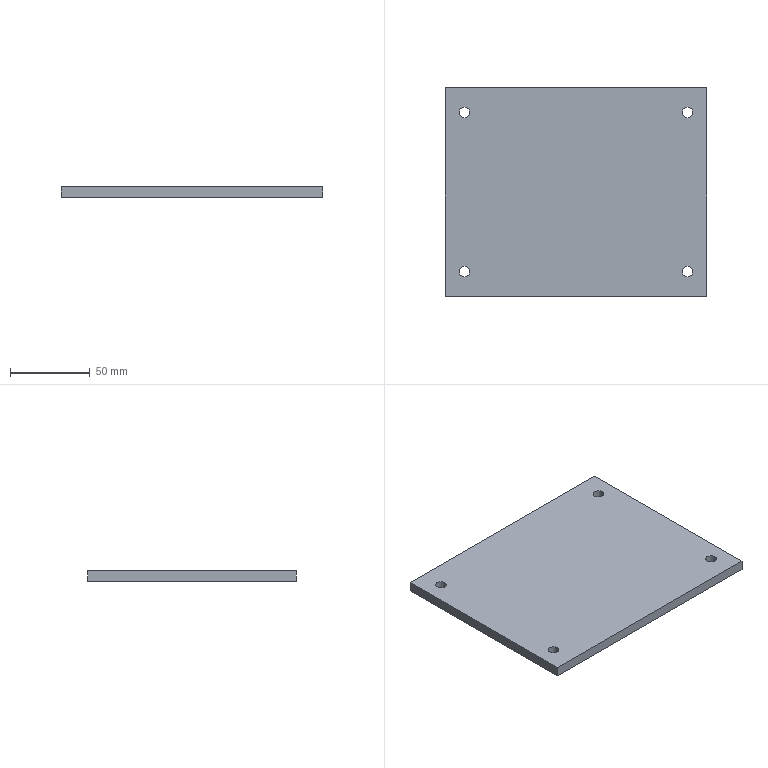Part | SolidWorks | features BaseBody 1 | 1 solid | 14 faces | box 164 x 131 x 6.4 mm | volume 136609 mm3 | cylinder 8 | plane 6 | commonest cylinder face diameters 6.647 x8
STEP:
#1=CARTESIAN_POINT('',(3.323,99.5,0.));
#2=VERTEX_POINT('',#1);
#3=CARTESIAN_POINT('',(-3.324,99.5,0.));
#4=VERTEX_POINT('',#3);
#5=CARTESIAN_POINT('',(0.,99.5,0.));
#6=DIRECTION('',(0.,0.,-1.));
#7=DIRECTION('',(1.,0.,0.));
#8=AXIS2_PLACEMENT_3D('',#5,#6,#7);
#9=CIRCLE('',#8,3.324);
#10=EDGE_CURVE('',#2,#4,#9,.T.);
#11=ORIENTED_EDGE('',*,*,#10,.T.);
#12=CARTESIAN_POINT('',(-3.324,99.5,6.4));
#13=VERTEX_POINT('',#12);
#14=CARTESIAN_POINT('',(-3.324,99.5,-203.595));
#15=DIRECTION('',(0.,0.,1.));
#16=VECTOR('',#15,1000.);
#17=LINE('',#14,#16);
#18=EDGE_CURVE('',#4,#13,#17,.T.);
#19=ORIENTED_EDGE('',*,*,#18,.T.);
#20=CARTESIAN_POINT('',(3.323,99.5,6.4));
#21=VERTEX_POINT('',#20);
#22=CARTESIAN_POINT('',(0.,99.5,6.4));
#23=DIRECTION('',(0.,0.,-1.));
#24=DIRECTION('',(1.,0.,0.));
#25=AXIS2_PLACEMENT_3D('',#22,#23,#24);
#26=CIRCLE('',#25,3.324);
#27=EDGE_CURVE('',#21,#13,#26,.T.);
#28=ORIENTED_EDGE('',*,*,#27,.F.);
#29=CARTESIAN_POINT('',(3.323,99.5,-203.595));
#30=DIRECTION('',(0.,0.,1.));
#31=VECTOR('',#30,1000.);
#32=LINE('',#29,#31);
#33=EDGE_CURVE('',#2,#21,#32,.T.);
#34=ORIENTED_EDGE('',*,*,#33,.F.);
#35=EDGE_LOOP('',(#11,#19,#28,#34));
#36=FACE_OUTER_BOUND('',#35,.T.);
#37=CARTESIAN_POINT('',(0.,99.5,-203.595));
#38=DIRECTION('',(0.,0.,1.));
#39=DIRECTION('',(1.,0.,0.));
#40=AXIS2_PLACEMENT_3D('',#37,#38,#39);
#41=CYLINDRICAL_SURFACE('',#40,3.324);
#42=ADVANCED_FACE('',(#36),#41,.F.);
#43=CARTESIAN_POINT('',(3.323,-0.5,0.));
#44=VERTEX_POINT('',#43);
#45=CARTESIAN_POINT('',(-3.324,-0.5,0.));
#46=VERTEX_POINT('',#45);
#47=CARTESIAN_POINT('',(0.,-0.5,0.));
#48=DIRECTION('',(0.,0.,-1.));
#49=DIRECTION('',(1.,0.,0.));
#50=AXIS2_PLACEMENT_3D('',#47,#48,#49);
#51=CIRCLE('',#50,3.324);
#52=EDGE_CURVE('',#44,#46,#51,.T.);
#53=ORIENTED_EDGE('',*,*,#52,.T.);
#54=CARTESIAN_POINT('',(-3.324,-0.5,6.4));
#55=VERTEX_POINT('',#54);
#56=CARTESIAN_POINT('',(-3.324,-0.5,-203.595));
#57=DIRECTION('',(0.,0.,1.));
#58=VECTOR('',#57,1000.);
#59=LINE('',#56,#58);
#60=EDGE_CURVE('',#46,#55,#59,.T.);
#61=ORIENTED_EDGE('',*,*,#60,.T.);
#62=CARTESIAN_POINT('',(3.323,-0.5,6.4));
#63=VERTEX_POINT('',#62);
#64=CARTESIAN_POINT('',(0.,-0.5,6.4));
#65=DIRECTION('',(0.,0.,-1.));
#66=DIRECTION('',(1.,0.,0.));
#67=AXIS2_PLACEMENT_3D('',#64,#65,#66);
#68=CIRCLE('',#67,3.324);
#69=EDGE_CURVE('',#63,#55,#68,.T.);
#70=ORIENTED_EDGE('',*,*,#69,.F.);
#71=CARTESIAN_POINT('',(3.323,-0.5,-203.595));
#72=DIRECTION('',(0.,0.,1.));
#73=VECTOR('',#72,1000.);
#74=LINE('',#71,#73);
#75=EDGE_CURVE('',#44,#63,#74,.T.);
#76=ORIENTED_EDGE('',*,*,#75,.F.);
#77=EDGE_LOOP('',(#53,#61,#70,#76));
#78=FACE_OUTER_BOUND('',#77,.T.);
#79=CARTESIAN_POINT('',(0.,-0.5,-203.595));
#80=DIRECTION('',(0.,0.,1.));
#81=DIRECTION('',(1.,0.,0.));
#82=AXIS2_PLACEMENT_3D('',#79,#80,#81);
#83=CYLINDRICAL_SURFACE('',#82,3.324);
#84=ADVANCED_FACE('',(#78),#83,.F.);
#85=CARTESIAN_POINT('',(143.324,-0.5,0.));
#86=VERTEX_POINT('',#85);
#87=CARTESIAN_POINT('',(136.677,-0.5,0.));
#88=VERTEX_POINT('',#87);
#89=CARTESIAN_POINT('',(140.,-0.5,0.));
#90=DIRECTION('',(0.,0.,-1.));
#91=DIRECTION('',(1.,0.,0.));
#92=AXIS2_PLACEMENT_3D('',#89,#90,#91);
#93=CIRCLE('',#92,3.324);
#94=EDGE_CURVE('',#86,#88,#93,.T.);
#95=ORIENTED_EDGE('',*,*,#94,.T.);
#96=CARTESIAN_POINT('',(136.677,-0.5,6.4));
#97=VERTEX_POINT('',#96);
#98=CARTESIAN_POINT('',(136.677,-0.5,-203.595));
#99=DIRECTION('',(0.,0.,1.));
#100=VECTOR('',#99,1000.);
#101=LINE('',#98,#100);
#102=EDGE_CURVE('',#88,#97,#101,.T.);
#103=ORIENTED_EDGE('',*,*,#102,.T.);
#104=CARTESIAN_POINT('',(143.324,-0.5,6.4));
#105=VERTEX_POINT('',#104);
#106=CARTESIAN_POINT('',(140.,-0.5,6.4));
#107=DIRECTION('',(0.,0.,-1.));
#108=DIRECTION('',(1.,0.,0.));
#109=AXIS2_PLACEMENT_3D('',#106,#107,#108);
#110=CIRCLE('',#109,3.324);
#111=EDGE_CURVE('',#105,#97,#110,.T.);
#112=ORIENTED_EDGE('',*,*,#111,.F.);
#113=CARTESIAN_POINT('',(143.324,-0.5,-203.595));
#114=DIRECTION('',(0.,0.,1.));
#115=VECTOR('',#114,1000.);
#116=LINE('',#113,#115);
#117=EDGE_CURVE('',#86,#105,#116,.T.);
#118=ORIENTED_EDGE('',*,*,#117,.F.);
#119=EDGE_LOOP('',(#95,#103,#112,#118));
#120=FACE_OUTER_BOUND('',#119,.T.);
#121=CARTESIAN_POINT('',(140.,-0.5,-203.595));
#122=DIRECTION('',(0.,0.,1.));
#123=DIRECTION('',(1.,0.,0.));
#124=AXIS2_PLACEMENT_3D('',#121,#122,#123);
#125=CYLINDRICAL_SURFACE('',#124,3.324);
#126=ADVANCED_FACE('',(#120),#125,.F.);
#127=CARTESIAN_POINT('',(143.324,99.5,0.));
#128=VERTEX_POINT('',#127);
#129=CARTESIAN_POINT('',(136.677,99.5,0.));
#130=VERTEX_POINT('',#129);
#131=CARTESIAN_POINT('',(140.,99.5,0.));
#132=DIRECTION('',(0.,0.,-1.));
#133=DIRECTION('',(1.,0.,0.));
#134=AXIS2_PLACEMENT_3D('',#131,#132,#133);
#135=CIRCLE('',#134,3.324);
#136=EDGE_CURVE('',#128,#130,#135,.T.);
#137=ORIENTED_EDGE('',*,*,#136,.T.);
#138=CARTESIAN_POINT('',(136.677,99.5,6.4));
#139=VERTEX_POINT('',#138);
#140=CARTESIAN_POINT('',(136.677,99.5,-203.595));
#141=DIRECTION('',(0.,0.,1.));
#142=VECTOR('',#141,1000.);
#143=LINE('',#140,#142);
#144=EDGE_CURVE('',#130,#139,#143,.T.);
#145=ORIENTED_EDGE('',*,*,#144,.T.);
#146=CARTESIAN_POINT('',(143.324,99.5,6.4));
#147=VERTEX_POINT('',#146);
#148=CARTESIAN_POINT('',(140.,99.5,6.4));
#149=DIRECTION('',(0.,0.,-1.));
#150=DIRECTION('',(1.,0.,0.));
#151=AXIS2_PLACEMENT_3D('',#148,#149,#150);
#152=CIRCLE('',#151,3.324);
#153=EDGE_CURVE('',#147,#139,#152,.T.);
#154=ORIENTED_EDGE('',*,*,#153,.F.);
#155=CARTESIAN_POINT('',(143.324,99.5,-203.595));
#156=DIRECTION('',(0.,0.,1.));
#157=VECTOR('',#156,1000.);
#158=LINE('',#155,#157);
#159=EDGE_CURVE('',#128,#147,#158,.T.);
#160=ORIENTED_EDGE('',*,*,#159,.F.);
#161=EDGE_LOOP('',(#137,#145,#154,#160));
#162=FACE_OUTER_BOUND('',#161,.T.);
#163=CARTESIAN_POINT('',(140.,99.5,-203.595));
#164=DIRECTION('',(0.,0.,1.));
#165=DIRECTION('',(1.,0.,0.));
#166=AXIS2_PLACEMENT_3D('',#163,#164,#165);
#167=CYLINDRICAL_SURFACE('',#166,3.324);
#168=ADVANCED_FACE('',(#162),#167,.F.);
#169=ORIENTED_EDGE('',*,*,#10,.F.);
#170=CARTESIAN_POINT('',(0.,99.5,0.));
#171=DIRECTION('',(0.,0.,-1.));
#172=DIRECTION('',(1.,0.,0.));
#173=AXIS2_PLACEMENT_3D('',#170,#171,#172);
#174=CIRCLE('',#173,3.324);
#175=EDGE_CURVE('',#4,#2,#174,.T.);
#176=ORIENTED_EDGE('',*,*,#175,.F.);
#177=EDGE_LOOP('',(#169,#176));
#178=FACE_BOUND('',#177,.T.);
#179=ORIENTED_EDGE('',*,*,#52,.F.);
#180=CARTESIAN_POINT('',(0.,-0.5,0.));
#181=DIRECTION('',(0.,0.,-1.));
#182=DIRECTION('',(1.,0.,0.));
#183=AXIS2_PLACEMENT_3D('',#180,#181,#182);
#184=CIRCLE('',#183,3.324);
#185=EDGE_CURVE('',#46,#44,#184,.T.);
#186=ORIENTED_EDGE('',*,*,#185,.F.);
#187=EDGE_LOOP('',(#179,#186));
#188=FACE_BOUND('',#187,.T.);
#189=ORIENTED_EDGE('',*,*,#94,.F.);
#190=CARTESIAN_POINT('',(140.,-0.5,0.));
#191=DIRECTION('',(0.,0.,-1.));
#192=DIRECTION('',(1.,0.,0.));
#193=AXIS2_PLACEMENT_3D('',#190,#191,#192);
#194=CIRCLE('',#193,3.324);
#195=EDGE_CURVE('',#88,#86,#194,.T.);
#196=ORIENTED_EDGE('',*,*,#195,.F.);
#197=EDGE_LOOP('',(#189,#196));
#198=FACE_BOUND('',#197,.T.);
#199=ORIENTED_EDGE('',*,*,#136,.F.);
#200=CARTESIAN_POINT('',(140.,99.5,0.));
#201=DIRECTION('',(0.,0.,-1.));
#202=DIRECTION('',(1.,0.,0.));
#203=AXIS2_PLACEMENT_3D('',#200,#201,#202);
#204=CIRCLE('',#203,3.324);
#205=EDGE_CURVE('',#130,#128,#204,.T.);
#206=ORIENTED_EDGE('',*,*,#205,.F.);
#207=EDGE_LOOP('',(#199,#206));
#208=FACE_BOUND('',#207,.T.);
#209=CARTESIAN_POINT('',(152.,-16.,0.));
#210=VERTEX_POINT('',#209);
#211=CARTESIAN_POINT('',(152.,115.,0.));
#212=VERTEX_POINT('',#211);
#213=CARTESIAN_POINT('',(152.,49.5,0.));
#214=DIRECTION('',(0.,1.,0.));
#215=VECTOR('',#214,1000.);
#216=LINE('',#213,#215);
#217=EDGE_CURVE('',#210,#212,#216,.T.);
#218=ORIENTED_EDGE('',*,*,#217,.F.);
#219=CARTESIAN_POINT('',(-12.,-16.,0.));
#220=VERTEX_POINT('',#219);
#221=CARTESIAN_POINT('',(70.,-16.,0.));
#222=DIRECTION('',(1.,0.,0.));
#223=VECTOR('',#222,1000.);
#224=LINE('',#221,#223);
#225=EDGE_CURVE('',#220,#210,#224,.T.);
#226=ORIENTED_EDGE('',*,*,#225,.F.);
#227=CARTESIAN_POINT('',(-12.,115.,0.));
#228=VERTEX_POINT('',#227);
#229=CARTESIAN_POINT('',(-12.,49.5,0.));
#230=DIRECTION('',(0.,-1.,0.));
#231=VECTOR('',#230,1000.);
#232=LINE('',#229,#231);
#233=EDGE_CURVE('',#228,#220,#232,.T.);
#234=ORIENTED_EDGE('',*,*,#233,.F.);
#235=CARTESIAN_POINT('',(70.,115.,0.));
#236=DIRECTION('',(-1.,0.,0.));
#237=VECTOR('',#236,1000.);
#238=LINE('',#235,#237);
#239=EDGE_CURVE('',#212,#228,#238,.T.);
#240=ORIENTED_EDGE('',*,*,#239,.F.);
#241=EDGE_LOOP('',(#218,#226,#234,#240));
#242=FACE_OUTER_BOUND('',#241,.T.);
#243=CARTESIAN_POINT('',(70.,49.5,0.));
#244=DIRECTION('',(0.,0.,1.));
#245=DIRECTION('',(1.,0.,0.));
#246=AXIS2_PLACEMENT_3D('',#243,#244,#245);
#247=PLANE('',#246);
#248=ADVANCED_FACE('',(#178,#188,#198,#208,#242),#247,.F.);
#249=ORIENTED_EDGE('',*,*,#18,.F.);
#250=ORIENTED_EDGE('',*,*,#175,.T.);
#251=ORIENTED_EDGE('',*,*,#33,.T.);
#252=CARTESIAN_POINT('',(0.,99.5,6.4));
#253=DIRECTION('',(0.,0.,-1.));
#254=DIRECTION('',(1.,0.,0.));
#255=AXIS2_PLACEMENT_3D('',#252,#253,#254);
#256=CIRCLE('',#255,3.324);
#257=EDGE_CURVE('',#13,#21,#256,.T.);
#258=ORIENTED_EDGE('',*,*,#257,.F.);
#259=EDGE_LOOP('',(#249,#250,#251,#258));
#260=FACE_OUTER_BOUND('',#259,.T.);
#261=CARTESIAN_POINT('',(0.,99.5,-203.595));
#262=DIRECTION('',(0.,0.,1.));
#263=DIRECTION('',(1.,0.,0.));
#264=AXIS2_PLACEMENT_3D('',#261,#262,#263);
#265=CYLINDRICAL_SURFACE('',#264,3.324);
#266=ADVANCED_FACE('',(#260),#265,.F.);
#267=ORIENTED_EDGE('',*,*,#60,.F.);
#268=ORIENTED_EDGE('',*,*,#185,.T.);
#269=ORIENTED_EDGE('',*,*,#75,.T.);
#270=CARTESIAN_POINT('',(0.,-0.5,6.4));
#271=DIRECTION('',(0.,0.,-1.));
#272=DIRECTION('',(1.,0.,0.));
#273=AXIS2_PLACEMENT_3D('',#270,#271,#272);
#274=CIRCLE('',#273,3.324);
#275=EDGE_CURVE('',#55,#63,#274,.T.);
#276=ORIENTED_EDGE('',*,*,#275,.F.);
#277=EDGE_LOOP('',(#267,#268,#269,#276));
#278=FACE_OUTER_BOUND('',#277,.T.);
#279=CARTESIAN_POINT('',(0.,-0.5,-203.595));
#280=DIRECTION('',(0.,0.,1.));
#281=DIRECTION('',(1.,0.,0.));
#282=AXIS2_PLACEMENT_3D('',#279,#280,#281);
#283=CYLINDRICAL_SURFACE('',#282,3.324);
#284=ADVANCED_FACE('',(#278),#283,.F.);
#285=ORIENTED_EDGE('',*,*,#102,.F.);
#286=ORIENTED_EDGE('',*,*,#195,.T.);
#287=ORIENTED_EDGE('',*,*,#117,.T.);
#288=CARTESIAN_POINT('',(140.,-0.5,6.4));
#289=DIRECTION('',(0.,0.,-1.));
#290=DIRECTION('',(1.,0.,0.));
#291=AXIS2_PLACEMENT_3D('',#288,#289,#290);
#292=CIRCLE('',#291,3.324);
#293=EDGE_CURVE('',#97,#105,#292,.T.);
#294=ORIENTED_EDGE('',*,*,#293,.F.);
#295=EDGE_LOOP('',(#285,#286,#287,#294));
#296=FACE_OUTER_BOUND('',#295,.T.);
#297=CARTESIAN_POINT('',(140.,-0.5,-203.595));
#298=DIRECTION('',(0.,0.,1.));
#299=DIRECTION('',(1.,0.,0.));
#300=AXIS2_PLACEMENT_3D('',#297,#298,#299);
#301=CYLINDRICAL_SURFACE('',#300,3.324);
#302=ADVANCED_FACE('',(#296),#301,.F.);
#303=ORIENTED_EDGE('',*,*,#144,.F.);
#304=ORIENTED_EDGE('',*,*,#205,.T.);
#305=ORIENTED_EDGE('',*,*,#159,.T.);
#306=CARTESIAN_POINT('',(140.,99.5,6.4));
#307=DIRECTION('',(0.,0.,-1.));
#308=DIRECTION('',(1.,0.,0.));
#309=AXIS2_PLACEMENT_3D('',#306,#307,#308);
#310=CIRCLE('',#309,3.324);
#311=EDGE_CURVE('',#139,#147,#310,.T.);
#312=ORIENTED_EDGE('',*,*,#311,.F.);
#313=EDGE_LOOP('',(#303,#304,#305,#312));
#314=FACE_OUTER_BOUND('',#313,.T.);
#315=CARTESIAN_POINT('',(140.,99.5,-203.595));
#316=DIRECTION('',(0.,0.,1.));
#317=DIRECTION('',(1.,0.,0.));
#318=AXIS2_PLACEMENT_3D('',#315,#316,#317);
#319=CYLINDRICAL_SURFACE('',#318,3.324);
#320=ADVANCED_FACE('',(#314),#319,.F.);
#321=ORIENTED_EDGE('',*,*,#239,.T.);
#322=CARTESIAN_POINT('',(-12.,115.,6.4));
#323=VERTEX_POINT('',#322);
#324=CARTESIAN_POINT('',(-12.,115.,0.));
#325=DIRECTION('',(0.,0.,1.));
#326=VECTOR('',#325,1000.);
#327=LINE('',#324,#326);
#328=EDGE_CURVE('',#228,#323,#327,.T.);
#329=ORIENTED_EDGE('',*,*,#328,.T.);
#330=CARTESIAN_POINT('',(152.,115.,6.4));
#331=VERTEX_POINT('',#330);
#332=CARTESIAN_POINT('',(-12.,115.,6.4));
#333=DIRECTION('',(1.,0.,0.));
#334=VECTOR('',#333,1000.);
#335=LINE('',#332,#334);
#336=EDGE_CURVE('',#323,#331,#335,.T.);
#337=ORIENTED_EDGE('',*,*,#336,.T.);
#338=CARTESIAN_POINT('',(152.,115.,0.));
#339=DIRECTION('',(0.,0.,-1.));
#340=VECTOR('',#339,1000.);
#341=LINE('',#338,#340);
#342=EDGE_CURVE('',#331,#212,#341,.T.);
#343=ORIENTED_EDGE('',*,*,#342,.T.);
#344=EDGE_LOOP('',(#321,#329,#337,#343));
#345=FACE_OUTER_BOUND('',#344,.T.);
#346=CARTESIAN_POINT('',(-12.,115.,0.));
#347=DIRECTION('',(0.,1.,0.));
#348=DIRECTION('',(0.,0.,1.));
#349=AXIS2_PLACEMENT_3D('',#346,#347,#348);
#350=PLANE('',#349);
#351=ADVANCED_FACE('',(#345),#350,.T.);
#352=ORIENTED_EDGE('',*,*,#217,.T.);
#353=ORIENTED_EDGE('',*,*,#342,.F.);
#354=CARTESIAN_POINT('',(152.,-16.,6.4));
#355=VERTEX_POINT('',#354);
#356=CARTESIAN_POINT('',(152.,115.,6.4));
#357=DIRECTION('',(0.,-1.,0.));
#358=VECTOR('',#357,1000.);
#359=LINE('',#356,#358);
#360=EDGE_CURVE('',#331,#355,#359,.T.);
#361=ORIENTED_EDGE('',*,*,#360,.T.);
#362=CARTESIAN_POINT('',(152.,-16.,0.));
#363=DIRECTION('',(0.,0.,-1.));
#364=VECTOR('',#363,1000.);
#365=LINE('',#362,#364);
#366=EDGE_CURVE('',#355,#210,#365,.T.);
#367=ORIENTED_EDGE('',*,*,#366,.T.);
#368=EDGE_LOOP('',(#352,#353,#361,#367));
#369=FACE_OUTER_BOUND('',#368,.T.);
#370=CARTESIAN_POINT('',(152.,115.,0.));
#371=DIRECTION('',(1.,0.,0.));
#372=DIRECTION('',(0.,0.,-1.));
#373=AXIS2_PLACEMENT_3D('',#370,#371,#372);
#374=PLANE('',#373);
#375=ADVANCED_FACE('',(#369),#374,.T.);
#376=ORIENTED_EDGE('',*,*,#225,.T.);
#377=ORIENTED_EDGE('',*,*,#366,.F.);
#378=CARTESIAN_POINT('',(-12.,-16.,6.4));
#379=VERTEX_POINT('',#378);
#380=CARTESIAN_POINT('',(152.,-16.,6.4));
#381=DIRECTION('',(-1.,0.,0.));
#382=VECTOR('',#381,1000.);
#383=LINE('',#380,#382);
#384=EDGE_CURVE('',#355,#379,#383,.T.);
#385=ORIENTED_EDGE('',*,*,#384,.T.);
#386=CARTESIAN_POINT('',(-12.,-16.,0.));
#387=DIRECTION('',(0.,0.,-1.));
#388=VECTOR('',#387,1000.);
#389=LINE('',#386,#388);
#390=EDGE_CURVE('',#379,#220,#389,.T.);
#391=ORIENTED_EDGE('',*,*,#390,.T.);
#392=EDGE_LOOP('',(#376,#377,#385,#391));
#393=FACE_OUTER_BOUND('',#392,.T.);
#394=CARTESIAN_POINT('',(152.,-16.,0.));
#395=DIRECTION('',(0.,-1.,0.));
#396=DIRECTION('',(1.,0.,0.));
#397=AXIS2_PLACEMENT_3D('',#394,#395,#396);
#398=PLANE('',#397);
#399=ADVANCED_FACE('',(#393),#398,.T.);
#400=ORIENTED_EDGE('',*,*,#233,.T.);
#401=ORIENTED_EDGE('',*,*,#390,.F.);
#402=CARTESIAN_POINT('',(-12.,-16.,6.4));
#403=DIRECTION('',(0.,1.,0.));
#404=VECTOR('',#403,1000.);
#405=LINE('',#402,#404);
#406=EDGE_CURVE('',#379,#323,#405,.T.);
#407=ORIENTED_EDGE('',*,*,#406,.T.);
#408=ORIENTED_EDGE('',*,*,#328,.F.);
#409=EDGE_LOOP('',(#400,#401,#407,#408));
#410=FACE_OUTER_BOUND('',#409,.T.);
#411=CARTESIAN_POINT('',(-12.,-16.,0.));
#412=DIRECTION('',(-1.,0.,0.));
#413=DIRECTION('',(0.,-1.,0.));
#414=AXIS2_PLACEMENT_3D('',#411,#412,#413);
#415=PLANE('',#414);
#416=ADVANCED_FACE('',(#410),#415,.T.);
#417=ORIENTED_EDGE('',*,*,#27,.T.);
#418=ORIENTED_EDGE('',*,*,#257,.T.);
#419=EDGE_LOOP('',(#417,#418));
#420=FACE_BOUND('',#419,.T.);
#421=ORIENTED_EDGE('',*,*,#69,.T.);
#422=ORIENTED_EDGE('',*,*,#275,.T.);
#423=EDGE_LOOP('',(#421,#422));
#424=FACE_BOUND('',#423,.T.);
#425=ORIENTED_EDGE('',*,*,#111,.T.);
#426=ORIENTED_EDGE('',*,*,#293,.T.);
#427=EDGE_LOOP('',(#425,#426));
#428=FACE_BOUND('',#427,.T.);
#429=ORIENTED_EDGE('',*,*,#153,.T.);
#430=ORIENTED_EDGE('',*,*,#311,.T.);
#431=EDGE_LOOP('',(#429,#430));
#432=FACE_BOUND('',#431,.T.);
#433=ORIENTED_EDGE('',*,*,#406,.F.);
#434=ORIENTED_EDGE('',*,*,#384,.F.);
#435=ORIENTED_EDGE('',*,*,#360,.F.);
#436=ORIENTED_EDGE('',*,*,#336,.F.);
#437=EDGE_LOOP('',(#433,#434,#435,#436));
#438=FACE_OUTER_BOUND('',#437,.T.);
#439=CARTESIAN_POINT('',(70.,49.5,6.4));
#440=DIRECTION('',(0.,0.,1.));
#441=DIRECTION('',(1.,0.,0.));
#442=AXIS2_PLACEMENT_3D('',#439,#440,#441);
#443=PLANE('',#442);
#444=ADVANCED_FACE('',(#420,#424,#428,#432,#438),#443,.T.);
#445=CLOSED_SHELL('',(#42,#84,#126,#168,#248,#266,#284,#302,#320,#351,#375,#399,#416,#444));
#446=MANIFOLD_SOLID_BREP('',#445);
#447=CARTESIAN_POINT('',(0.,0.,0.));
#448=DIRECTION('',(0.,0.,1.));
#449=DIRECTION('',(1.,0.,0.));
#450=AXIS2_PLACEMENT_3D('',#447,#448,#449);
#451=(LENGTH_UNIT()NAMED_UNIT(*)SI_UNIT(.MILLI.,.METRE.));
#452=UNCERTAINTY_MEASURE_WITH_UNIT(LENGTH_MEASURE(0.00001),#451,'','');
#453=(NAMED_UNIT(*)PLANE_ANGLE_UNIT()SI_UNIT($,.RADIAN.));
#454=(NAMED_UNIT(*)SI_UNIT($,.STERADIAN.)SOLID_ANGLE_UNIT());
#455=(GEOMETRIC_REPRESENTATION_CONTEXT(3)GLOBAL_UNCERTAINTY_ASSIGNED_CONTEXT((#452))GLOBAL_UNIT_ASSIGNED_CONTEXT((#451,#453,#454))REPRESENTATION_CONTEXT('',''));
#456=ADVANCED_BREP_SHAPE_REPRESENTATION('',(#446,#450),#455);